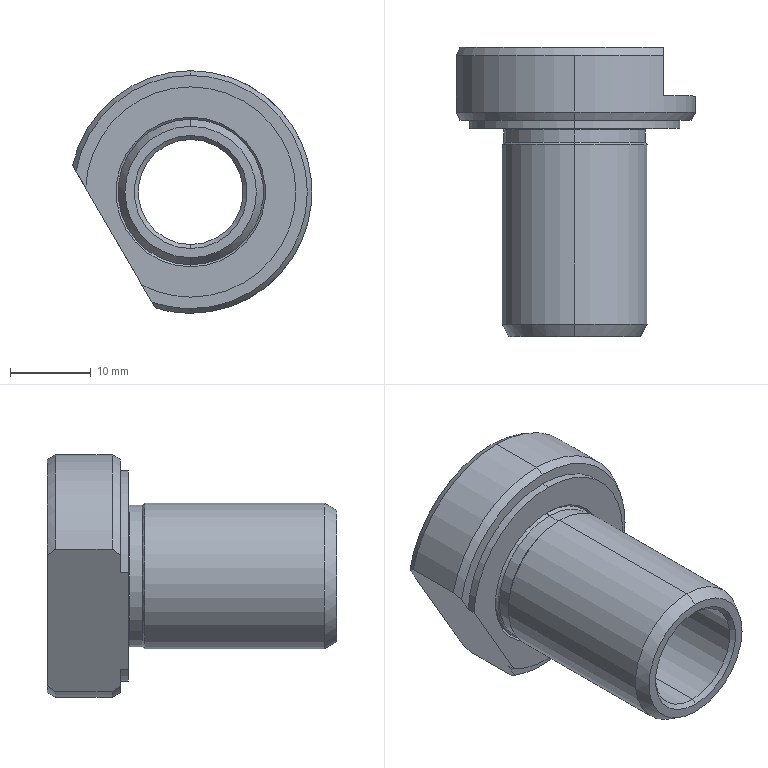Part | SolidWorks | features Chamfer 7, Cut 2, Fillet 1, Revolution 1 | 1 solid | 37 faces | box 29.63 x 35.75 x 30 mm | volume 7686 mm3 | cone 16 | cylinder 12 | plane 7 | torus 2 | commonest cylinder face diameters 26 x3 30 x3 13 x2 17.5 x2 18 x2
STEP:
#1=CARTESIAN_POINT('',(0.,-35.75,-8.134));
#2=VERTEX_POINT('',#1);
#3=CARTESIAN_POINT('',(0.,-35.75,8.134));
#4=VERTEX_POINT('',#3);
#5=CARTESIAN_POINT('',(0.,-35.75,0.));
#6=DIRECTION('',(0.,-1.,0.));
#7=DIRECTION('',(0.,0.,1.));
#8=AXIS2_PLACEMENT_3D('',#5,#6,#7);
#9=CIRCLE('',#8,8.134);
#10=EDGE_CURVE('',#2,#4,#9,.T.);
#11=ORIENTED_EDGE('',*,*,#10,.F.);
#12=CARTESIAN_POINT('',(0.,-34.25,-9.));
#13=VERTEX_POINT('',#12);
#14=CARTESIAN_POINT('',(0.,-34.25,-9.));
#15=DIRECTION('',(0.,0.866,-0.5));
#16=VECTOR('',#15,1000.);
#17=LINE('',#14,#16);
#18=EDGE_CURVE('',#2,#13,#17,.T.);
#19=ORIENTED_EDGE('',*,*,#18,.T.);
#20=CARTESIAN_POINT('',(0.,-34.25,9.));
#21=VERTEX_POINT('',#20);
#22=CARTESIAN_POINT('',(0.,-34.25,0.));
#23=DIRECTION('',(0.,1.,0.));
#24=DIRECTION('',(0.,0.,1.));
#25=AXIS2_PLACEMENT_3D('',#22,#23,#24);
#26=CIRCLE('',#25,9.);
#27=EDGE_CURVE('',#21,#13,#26,.T.);
#28=ORIENTED_EDGE('',*,*,#27,.F.);
#29=CARTESIAN_POINT('',(0.,-34.25,9.));
#30=DIRECTION('',(0.,0.866,0.5));
#31=VECTOR('',#30,1000.);
#32=LINE('',#29,#31);
#33=EDGE_CURVE('',#4,#21,#32,.T.);
#34=ORIENTED_EDGE('',*,*,#33,.F.);
#35=EDGE_LOOP('',(#11,#19,#28,#34));
#36=FACE_OUTER_BOUND('',#35,.T.);
#37=CARTESIAN_POINT('',(0.,-34.25,0.));
#38=DIRECTION('',(0.,1.,0.));
#39=DIRECTION('',(0.,0.,1.));
#40=AXIS2_PLACEMENT_3D('',#37,#38,#39);
#41=CONICAL_SURFACE('',#40,9.,0.5236);
#42=ADVANCED_FACE('',(#36),#41,.T.);
#43=CARTESIAN_POINT('',(0.,-9.75,-9.));
#44=VERTEX_POINT('',#43);
#45=CARTESIAN_POINT('',(0.,-9.75,9.));
#46=VERTEX_POINT('',#45);
#47=CARTESIAN_POINT('',(0.,-9.75,0.));
#48=DIRECTION('',(0.,1.,0.));
#49=DIRECTION('',(0.,0.,1.));
#50=AXIS2_PLACEMENT_3D('',#47,#48,#49);
#51=CIRCLE('',#50,9.);
#52=EDGE_CURVE('',#44,#46,#51,.T.);
#53=ORIENTED_EDGE('',*,*,#52,.F.);
#54=CARTESIAN_POINT('',(0.,-10.183,-8.75));
#55=VERTEX_POINT('',#54);
#56=CARTESIAN_POINT('',(0.,-10.183,-9.25));
#57=DIRECTION('',(1.,0.,0.));
#58=DIRECTION('',(0.,0.,-1.));
#59=AXIS2_PLACEMENT_3D('',#56,#57,#58);
#60=CIRCLE('',#59,0.5);
#61=EDGE_CURVE('',#44,#55,#60,.T.);
#62=ORIENTED_EDGE('',*,*,#61,.T.);
#63=CARTESIAN_POINT('',(0.,-10.183,8.75));
#64=VERTEX_POINT('',#63);
#65=CARTESIAN_POINT('',(0.,-10.183,0.));
#66=DIRECTION('',(0.,-1.,0.));
#67=DIRECTION('',(0.,0.,1.));
#68=AXIS2_PLACEMENT_3D('',#65,#66,#67);
#69=CIRCLE('',#68,8.75);
#70=EDGE_CURVE('',#64,#55,#69,.T.);
#71=ORIENTED_EDGE('',*,*,#70,.F.);
#72=CARTESIAN_POINT('',(0.,-10.183,9.25));
#73=DIRECTION('',(-1.,0.,0.));
#74=DIRECTION('',(0.,0.,1.));
#75=AXIS2_PLACEMENT_3D('',#72,#73,#74);
#76=CIRCLE('',#75,0.5);
#77=EDGE_CURVE('',#46,#64,#76,.T.);
#78=ORIENTED_EDGE('',*,*,#77,.F.);
#79=EDGE_LOOP('',(#53,#62,#71,#78));
#80=FACE_OUTER_BOUND('',#79,.T.);
#81=CARTESIAN_POINT('',(0.,-10.183,0.));
#82=DIRECTION('',(0.,1.,0.));
#83=DIRECTION('',(0.,0.,1.));
#84=AXIS2_PLACEMENT_3D('',#81,#82,#83);
#85=TOROIDAL_SURFACE('',#84,9.25,0.5);
#86=ADVANCED_FACE('',(#80),#85,.F.);
#87=ORIENTED_EDGE('',*,*,#52,.T.);
#88=CARTESIAN_POINT('',(0.,-10.,9.25));
#89=VERTEX_POINT('',#88);
#90=CARTESIAN_POINT('',(0.,-10.,9.25));
#91=DIRECTION('',(0.,-0.7071,0.7071));
#92=VECTOR('',#91,1000.);
#93=LINE('',#90,#92);
#94=EDGE_CURVE('',#46,#89,#93,.T.);
#95=ORIENTED_EDGE('',*,*,#94,.T.);
#96=CARTESIAN_POINT('',(0.,-10.,-9.25));
#97=VERTEX_POINT('',#96);
#98=CARTESIAN_POINT('',(0.,-10.,0.));
#99=DIRECTION('',(0.,1.,0.));
#100=DIRECTION('',(0.,0.,1.));
#101=AXIS2_PLACEMENT_3D('',#98,#99,#100);
#102=CIRCLE('',#101,9.25);
#103=EDGE_CURVE('',#97,#89,#102,.T.);
#104=ORIENTED_EDGE('',*,*,#103,.F.);
#105=CARTESIAN_POINT('',(0.,-10.,-9.25));
#106=DIRECTION('',(0.,-0.7071,-0.7071));
#107=VECTOR('',#106,1000.);
#108=LINE('',#105,#107);
#109=EDGE_CURVE('',#44,#97,#108,.T.);
#110=ORIENTED_EDGE('',*,*,#109,.F.);
#111=EDGE_LOOP('',(#87,#95,#104,#110));
#112=FACE_OUTER_BOUND('',#111,.T.);
#113=CARTESIAN_POINT('',(0.,-10.,0.));
#114=DIRECTION('',(0.,-1.,0.));
#115=DIRECTION('',(0.,0.,-1.));
#116=AXIS2_PLACEMENT_3D('',#113,#114,#115);
#117=CONICAL_SURFACE('',#116,9.25,0.7854);
#118=ADVANCED_FACE('',(#112),#117,.F.);
#119=CARTESIAN_POINT('',(0.,-11.75,8.75));
#120=VERTEX_POINT('',#119);
#121=CARTESIAN_POINT('',(0.,-11.75,-8.75));
#122=VERTEX_POINT('',#121);
#123=CARTESIAN_POINT('',(0.,-11.75,0.));
#124=DIRECTION('',(0.,1.,0.));
#125=DIRECTION('',(0.,0.,1.));
#126=AXIS2_PLACEMENT_3D('',#123,#124,#125);
#127=CIRCLE('',#126,8.75);
#128=EDGE_CURVE('',#120,#122,#127,.T.);
#129=ORIENTED_EDGE('',*,*,#128,.F.);
#130=CARTESIAN_POINT('',(0.,-12.,9.));
#131=VERTEX_POINT('',#130);
#132=CARTESIAN_POINT('',(0.,-11.75,8.75));
#133=DIRECTION('',(0.,-0.7071,0.7071));
#134=VECTOR('',#133,1000.);
#135=LINE('',#132,#134);
#136=EDGE_CURVE('',#120,#131,#135,.T.);
#137=ORIENTED_EDGE('',*,*,#136,.T.);
#138=CARTESIAN_POINT('',(0.,-12.,-9.));
#139=VERTEX_POINT('',#138);
#140=CARTESIAN_POINT('',(0.,-12.,0.));
#141=DIRECTION('',(0.,-1.,0.));
#142=DIRECTION('',(0.,0.,-1.));
#143=AXIS2_PLACEMENT_3D('',#140,#141,#142);
#144=CIRCLE('',#143,9.);
#145=EDGE_CURVE('',#139,#131,#144,.T.);
#146=ORIENTED_EDGE('',*,*,#145,.F.);
#147=CARTESIAN_POINT('',(0.,-11.75,-8.75));
#148=DIRECTION('',(0.,-0.7071,-0.7071));
#149=VECTOR('',#148,1000.);
#150=LINE('',#147,#149);
#151=EDGE_CURVE('',#122,#139,#150,.T.);
#152=ORIENTED_EDGE('',*,*,#151,.F.);
#153=EDGE_LOOP('',(#129,#137,#146,#152));
#154=FACE_OUTER_BOUND('',#153,.T.);
#155=CARTESIAN_POINT('',(0.,-11.75,0.));
#156=DIRECTION('',(0.,-1.,0.));
#157=DIRECTION('',(0.,0.,-1.));
#158=AXIS2_PLACEMENT_3D('',#155,#156,#157);
#159=CONICAL_SURFACE('',#158,8.75,0.7854);
#160=ADVANCED_FACE('',(#154),#159,.T.);
#161=CARTESIAN_POINT('',(0.,-35.25,6.5));
#162=VERTEX_POINT('',#161);
#163=CARTESIAN_POINT('',(0.,-35.25,-6.5));
#164=VERTEX_POINT('',#163);
#165=CARTESIAN_POINT('',(0.,-35.25,0.));
#166=DIRECTION('',(0.,-1.,0.));
#167=DIRECTION('',(0.,0.,1.));
#168=AXIS2_PLACEMENT_3D('',#165,#166,#167);
#169=CIRCLE('',#168,6.5);
#170=EDGE_CURVE('',#162,#164,#169,.T.);
#171=ORIENTED_EDGE('',*,*,#170,.F.);
#172=CARTESIAN_POINT('',(0.,-35.75,7.));
#173=VERTEX_POINT('',#172);
#174=CARTESIAN_POINT('',(0.,-35.75,7.));
#175=DIRECTION('',(0.,-0.7071,0.7071));
#176=VECTOR('',#175,1000.);
#177=LINE('',#174,#176);
#178=EDGE_CURVE('',#162,#173,#177,.T.);
#179=ORIENTED_EDGE('',*,*,#178,.T.);
#180=CARTESIAN_POINT('',(0.,-35.75,-7.));
#181=VERTEX_POINT('',#180);
#182=CARTESIAN_POINT('',(0.,-35.75,0.));
#183=DIRECTION('',(0.,1.,0.));
#184=DIRECTION('',(0.,0.,1.));
#185=AXIS2_PLACEMENT_3D('',#182,#183,#184);
#186=CIRCLE('',#185,7.);
#187=EDGE_CURVE('',#181,#173,#186,.T.);
#188=ORIENTED_EDGE('',*,*,#187,.F.);
#189=CARTESIAN_POINT('',(0.,-35.75,-7.));
#190=DIRECTION('',(0.,-0.7071,-0.7071));
#191=VECTOR('',#190,1000.);
#192=LINE('',#189,#191);
#193=EDGE_CURVE('',#164,#181,#192,.T.);
#194=ORIENTED_EDGE('',*,*,#193,.F.);
#195=EDGE_LOOP('',(#171,#179,#188,#194));
#196=FACE_OUTER_BOUND('',#195,.T.);
#197=CARTESIAN_POINT('',(0.,-35.75,0.));
#198=DIRECTION('',(0.,-1.,0.));
#199=DIRECTION('',(0.,0.,-1.));
#200=AXIS2_PLACEMENT_3D('',#197,#198,#199);
#201=CONICAL_SURFACE('',#200,7.,0.7854);
#202=ADVANCED_FACE('',(#196),#201,.F.);
#203=CARTESIAN_POINT('',(0.,-2.,-6.5));
#204=VERTEX_POINT('',#203);
#205=CARTESIAN_POINT('',(0.,-2.,6.5));
#206=VERTEX_POINT('',#205);
#207=CARTESIAN_POINT('',(0.,-2.,0.));
#208=DIRECTION('',(0.,1.,0.));
#209=DIRECTION('',(0.,0.,-1.));
#210=AXIS2_PLACEMENT_3D('',#207,#208,#209);
#211=CIRCLE('',#210,6.5);
#212=EDGE_CURVE('',#204,#206,#211,.T.);
#213=ORIENTED_EDGE('',*,*,#212,.F.);
#214=CARTESIAN_POINT('',(0.,0.,-7.655));
#215=VERTEX_POINT('',#214);
#216=CARTESIAN_POINT('',(0.,-2.,-6.5));
#217=DIRECTION('',(0.,0.866,-0.5));
#218=VECTOR('',#217,1000.);
#219=LINE('',#216,#218);
#220=EDGE_CURVE('',#204,#215,#219,.T.);
#221=ORIENTED_EDGE('',*,*,#220,.T.);
#222=CARTESIAN_POINT('',(0.,0.,7.655));
#223=VERTEX_POINT('',#222);
#224=CARTESIAN_POINT('',(0.,0.,0.));
#225=DIRECTION('',(0.,-1.,0.));
#226=DIRECTION('',(0.,0.,-1.));
#227=AXIS2_PLACEMENT_3D('',#224,#225,#226);
#228=CIRCLE('',#227,7.655);
#229=EDGE_CURVE('',#223,#215,#228,.T.);
#230=ORIENTED_EDGE('',*,*,#229,.F.);
#231=CARTESIAN_POINT('',(0.,-2.,6.5));
#232=DIRECTION('',(0.,0.866,0.5));
#233=VECTOR('',#232,1000.);
#234=LINE('',#231,#233);
#235=EDGE_CURVE('',#206,#223,#234,.T.);
#236=ORIENTED_EDGE('',*,*,#235,.F.);
#237=EDGE_LOOP('',(#213,#221,#230,#236));
#238=FACE_OUTER_BOUND('',#237,.T.);
#239=CARTESIAN_POINT('',(0.,-2.,0.));
#240=DIRECTION('',(0.,1.,0.));
#241=DIRECTION('',(0.,0.,1.));
#242=AXIS2_PLACEMENT_3D('',#239,#240,#241);
#243=CONICAL_SURFACE('',#242,6.5,0.5236);
#244=ADVANCED_FACE('',(#238),#243,.F.);
#245=ORIENTED_EDGE('',*,*,#170,.T.);
#246=CARTESIAN_POINT('',(0.,102.352,-6.5));
#247=DIRECTION('',(0.,1.,0.));
#248=VECTOR('',#247,1000.);
#249=LINE('',#246,#248);
#250=EDGE_CURVE('',#164,#204,#249,.T.);
#251=ORIENTED_EDGE('',*,*,#250,.T.);
#252=ORIENTED_EDGE('',*,*,#212,.T.);
#253=CARTESIAN_POINT('',(0.,102.352,6.5));
#254=DIRECTION('',(0.,1.,0.));
#255=VECTOR('',#254,1000.);
#256=LINE('',#253,#255);
#257=EDGE_CURVE('',#162,#206,#256,.T.);
#258=ORIENTED_EDGE('',*,*,#257,.F.);
#259=EDGE_LOOP('',(#245,#251,#252,#258));
#260=FACE_OUTER_BOUND('',#259,.T.);
#261=CARTESIAN_POINT('',(0.,102.352,0.));
#262=DIRECTION('',(0.,1.,0.));
#263=DIRECTION('',(0.,0.,1.));
#264=AXIS2_PLACEMENT_3D('',#261,#262,#263);
#265=CYLINDRICAL_SURFACE('',#264,6.5);
#266=ADVANCED_FACE('',(#260),#265,.F.);
#267=ORIENTED_EDGE('',*,*,#27,.T.);
#268=CARTESIAN_POINT('',(0.,102.352,-9.));
#269=DIRECTION('',(0.,1.,0.));
#270=VECTOR('',#269,1000.);
#271=LINE('',#268,#270);
#272=EDGE_CURVE('',#13,#139,#271,.T.);
#273=ORIENTED_EDGE('',*,*,#272,.T.);
#274=ORIENTED_EDGE('',*,*,#145,.T.);
#275=CARTESIAN_POINT('',(0.,102.352,9.));
#276=DIRECTION('',(0.,1.,0.));
#277=VECTOR('',#276,1000.);
#278=LINE('',#275,#277);
#279=EDGE_CURVE('',#21,#131,#278,.T.);
#280=ORIENTED_EDGE('',*,*,#279,.F.);
#281=EDGE_LOOP('',(#267,#273,#274,#280));
#282=FACE_OUTER_BOUND('',#281,.T.);
#283=CARTESIAN_POINT('',(0.,102.352,0.));
#284=DIRECTION('',(0.,1.,0.));
#285=DIRECTION('',(0.,0.,1.));
#286=AXIS2_PLACEMENT_3D('',#283,#284,#285);
#287=CYLINDRICAL_SURFACE('',#286,9.);
#288=ADVANCED_FACE('',(#282),#287,.T.);
#289=ORIENTED_EDGE('',*,*,#128,.T.);
#290=CARTESIAN_POINT('',(0.,102.352,-8.75));
#291=DIRECTION('',(0.,1.,0.));
#292=VECTOR('',#291,1000.);
#293=LINE('',#290,#292);
#294=EDGE_CURVE('',#122,#55,#293,.T.);
#295=ORIENTED_EDGE('',*,*,#294,.T.);
#296=CARTESIAN_POINT('',(0.,-10.183,0.));
#297=DIRECTION('',(0.,-1.,0.));
#298=DIRECTION('',(0.,0.,1.));
#299=AXIS2_PLACEMENT_3D('',#296,#297,#298);
#300=CIRCLE('',#299,8.75);
#301=EDGE_CURVE('',#55,#64,#300,.T.);
#302=ORIENTED_EDGE('',*,*,#301,.T.);
#303=CARTESIAN_POINT('',(0.,102.352,8.75));
#304=DIRECTION('',(0.,1.,0.));
#305=VECTOR('',#304,1000.);
#306=LINE('',#303,#305);
#307=EDGE_CURVE('',#120,#64,#306,.T.);
#308=ORIENTED_EDGE('',*,*,#307,.F.);
#309=EDGE_LOOP('',(#289,#295,#302,#308));
#310=FACE_OUTER_BOUND('',#309,.T.);
#311=CARTESIAN_POINT('',(0.,102.352,0.));
#312=DIRECTION('',(0.,1.,0.));
#313=DIRECTION('',(0.,0.,1.));
#314=AXIS2_PLACEMENT_3D('',#311,#312,#313);
#315=CYLINDRICAL_SURFACE('',#314,8.75);
#316=ADVANCED_FACE('',(#310),#315,.T.);
#317=CARTESIAN_POINT('',(0.,-9.,-14.423));
#318=VERTEX_POINT('',#317);
#319=CARTESIAN_POINT('',(0.,-9.,14.423));
#320=VERTEX_POINT('',#319);
#321=CARTESIAN_POINT('',(0.,-9.,0.));
#322=DIRECTION('',(0.,-1.,0.));
#323=DIRECTION('',(0.,0.,1.));
#324=AXIS2_PLACEMENT_3D('',#321,#322,#323);
#325=CIRCLE('',#324,14.423);
#326=EDGE_CURVE('',#318,#320,#325,.T.);
#327=ORIENTED_EDGE('',*,*,#326,.F.);
#328=CARTESIAN_POINT('',(0.,-8.,-15.));
#329=VERTEX_POINT('',#328);
#330=CARTESIAN_POINT('',(0.,-8.,-15.));
#331=DIRECTION('',(0.,0.866,-0.5));
#332=VECTOR('',#331,1000.);
#333=LINE('',#330,#332);
#334=EDGE_CURVE('',#318,#329,#333,.T.);
#335=ORIENTED_EDGE('',*,*,#334,.T.);
#336=CARTESIAN_POINT('',(0.,-8.,15.));
#337=VERTEX_POINT('',#336);
#338=CARTESIAN_POINT('',(0.,-8.,0.));
#339=DIRECTION('',(0.,1.,0.));
#340=DIRECTION('',(0.,0.,1.));
#341=AXIS2_PLACEMENT_3D('',#338,#339,#340);
#342=CIRCLE('',#341,15.);
#343=EDGE_CURVE('',#337,#329,#342,.T.);
#344=ORIENTED_EDGE('',*,*,#343,.F.);
#345=CARTESIAN_POINT('',(0.,-8.,15.));
#346=DIRECTION('',(0.,0.866,0.5));
#347=VECTOR('',#346,1000.);
#348=LINE('',#345,#347);
#349=EDGE_CURVE('',#320,#337,#348,.T.);
#350=ORIENTED_EDGE('',*,*,#349,.F.);
#351=EDGE_LOOP('',(#327,#335,#344,#350));
#352=FACE_OUTER_BOUND('',#351,.T.);
#353=CARTESIAN_POINT('',(0.,-8.,0.));
#354=DIRECTION('',(0.,1.,0.));
#355=DIRECTION('',(0.,0.,1.));
#356=AXIS2_PLACEMENT_3D('',#353,#354,#355);
#357=CONICAL_SURFACE('',#356,15.,0.5236);
#358=ADVANCED_FACE('',(#352),#357,.T.);
#359=CARTESIAN_POINT('',(-14.194,-9.,2.56));
#360=VERTEX_POINT('',#359);
#361=CARTESIAN_POINT('',(0.,-9.,0.));
#362=DIRECTION('',(0.,-1.,0.));
#363=DIRECTION('',(0.,0.,1.));
#364=AXIS2_PLACEMENT_3D('',#361,#362,#363);
#365=CIRCLE('',#364,14.423);
#366=EDGE_CURVE('',#320,#360,#365,.T.);
#367=ORIENTED_EDGE('',*,*,#366,.F.);
#368=ORIENTED_EDGE('',*,*,#349,.T.);
#369=CARTESIAN_POINT('',(-14.63,-8.,3.313));
#370=VERTEX_POINT('',#369);
#371=CARTESIAN_POINT('',(0.,-8.,0.));
#372=DIRECTION('',(0.,1.,0.));
#373=DIRECTION('',(0.,0.,1.));
#374=AXIS2_PLACEMENT_3D('',#371,#372,#373);
#375=CIRCLE('',#374,15.);
#376=EDGE_CURVE('',#370,#337,#375,.T.);
#377=ORIENTED_EDGE('',*,*,#376,.F.);
#378=CARTESIAN_POINT('',(-14.63,-8.,3.313));
#379=CARTESIAN_POINT('',(-14.486,-8.337,3.065));
#380=CARTESIAN_POINT('',(-14.341,-8.67,2.815));
#381=CARTESIAN_POINT('',(-14.194,-9.,2.56));
#382=B_SPLINE_CURVE_WITH_KNOTS('',3,(#378,#379,#380,#381),.UNSPECIFIED.,.F.,.F.,(4,4),(0.03086,0.03219),.UNSPECIFIED.);
#383=EDGE_CURVE('',#370,#360,#382,.T.);
#384=ORIENTED_EDGE('',*,*,#383,.T.);
#385=EDGE_LOOP('',(#367,#368,#377,#384));
#386=FACE_OUTER_BOUND('',#385,.T.);
#387=CARTESIAN_POINT('',(0.,-8.,0.));
#388=DIRECTION('',(0.,1.,0.));
#389=DIRECTION('',(0.,0.,1.));
#390=AXIS2_PLACEMENT_3D('',#387,#388,#389);
#391=CONICAL_SURFACE('',#390,15.,0.5236);
#392=ADVANCED_FACE('',(#386),#391,.T.);
#393=CARTESIAN_POINT('',(0.,-10.,13.));
#394=VERTEX_POINT('',#393);
#395=CARTESIAN_POINT('',(0.,-10.,-13.));
#396=VERTEX_POINT('',#395);
#397=CARTESIAN_POINT('',(0.,-10.,0.));
#398=DIRECTION('',(0.,1.,0.));
#399=DIRECTION('',(0.,0.,1.));
#400=AXIS2_PLACEMENT_3D('',#397,#398,#399);
#401=CIRCLE('',#400,13.);
#402=EDGE_CURVE('',#394,#396,#401,.T.);
#403=ORIENTED_EDGE('',*,*,#402,.T.);
#404=CARTESIAN_POINT('',(0.,-9.,-13.));
#405=VERTEX_POINT('',#404);
#406=CARTESIAN_POINT('',(0.,102.352,-13.));
#407=DIRECTION('',(0.,1.,0.));
#408=VECTOR('',#407,1000.);
#409=LINE('',#406,#408);
#410=EDGE_CURVE('',#396,#405,#409,.T.);
#411=ORIENTED_EDGE('',*,*,#410,.T.);
#412=CARTESIAN_POINT('',(0.,-9.,13.));
#413=VERTEX_POINT('',#412);
#414=CARTESIAN_POINT('',(0.,-9.,0.));
#415=DIRECTION('',(0.,1.,0.));
#416=DIRECTION('',(0.,0.,1.));
#417=AXIS2_PLACEMENT_3D('',#414,#415,#416);
#418=CIRCLE('',#417,13.);
#419=EDGE_CURVE('',#413,#405,#418,.T.);
#420=ORIENTED_EDGE('',*,*,#419,.F.);
#421=CARTESIAN_POINT('',(0.,102.352,13.));
#422=DIRECTION('',(0.,1.,0.));
#423=VECTOR('',#422,1000.);
#424=LINE('',#421,#423);
#425=EDGE_CURVE('',#394,#413,#424,.T.);
#426=ORIENTED_EDGE('',*,*,#425,.F.);
#427=EDGE_LOOP('',(#403,#411,#420,#426));
#428=FACE_OUTER_BOUND('',#427,.T.);
#429=CARTESIAN_POINT('',(0.,102.352,0.));
#430=DIRECTION('',(0.,1.,0.));
#431=DIRECTION('',(0.,0.,1.));
#432=AXIS2_PLACEMENT_3D('',#429,#430,#431);
#433=CYLINDRICAL_SURFACE('',#432,13.);
#434=ADVANCED_FACE('',(#428),#433,.T.);
#435=CARTESIAN_POINT('',(-12.991,-10.,0.4832));
#436=VERTEX_POINT('',#435);
#437=CARTESIAN_POINT('',(0.,-10.,0.));
#438=DIRECTION('',(0.,1.,0.));
#439=DIRECTION('',(0.,0.,1.));
#440=AXIS2_PLACEMENT_3D('',#437,#438,#439);
#441=CIRCLE('',#440,13.);
#442=EDGE_CURVE('',#436,#394,#441,.T.);
#443=ORIENTED_EDGE('',*,*,#442,.T.);
#444=ORIENTED_EDGE('',*,*,#425,.T.);
#445=CARTESIAN_POINT('',(-12.991,-9.,0.4832));
#446=VERTEX_POINT('',#445);
#447=CARTESIAN_POINT('',(0.,-9.,0.));
#448=DIRECTION('',(0.,1.,0.));
#449=DIRECTION('',(0.,0.,1.));
#450=AXIS2_PLACEMENT_3D('',#447,#448,#449);
#451=CIRCLE('',#450,13.);
#452=EDGE_CURVE('',#446,#413,#451,.T.);
#453=ORIENTED_EDGE('',*,*,#452,.F.);
#454=CARTESIAN_POINT('',(-12.991,102.352,0.4832));
#455=DIRECTION('',(0.,1.,0.));
#456=VECTOR('',#455,1000.);
#457=LINE('',#454,#456);
#458=EDGE_CURVE('',#436,#446,#457,.T.);
#459=ORIENTED_EDGE('',*,*,#458,.F.);
#460=EDGE_LOOP('',(#443,#444,#453,#459));
#461=FACE_OUTER_BOUND('',#460,.T.);
#462=CARTESIAN_POINT('',(0.,102.352,0.));
#463=DIRECTION('',(0.,1.,0.));
#464=DIRECTION('',(0.,0.,1.));
#465=AXIS2_PLACEMENT_3D('',#462,#463,#464);
#466=CYLINDRICAL_SURFACE('',#465,13.);
#467=ADVANCED_FACE('',(#461),#466,.T.);
#468=CARTESIAN_POINT('',(0.,0.,-14.423));
#469=VERTEX_POINT('',#468);
#470=CARTESIAN_POINT('',(-4.845,0.,-13.585));
#471=VERTEX_POINT('',#470);
#472=CARTESIAN_POINT('',(0.,0.,0.));
#473=DIRECTION('',(0.,1.,0.));
#474=DIRECTION('',(0.,0.,-1.));
#475=AXIS2_PLACEMENT_3D('',#472,#473,#474);
#476=CIRCLE('',#475,14.423);
#477=EDGE_CURVE('',#469,#471,#476,.T.);
#478=ORIENTED_EDGE('',*,*,#477,.F.);
#479=CARTESIAN_POINT('',(0.,-1.,-15.));
#480=VERTEX_POINT('',#479);
#481=CARTESIAN_POINT('',(0.,0.,-14.423));
#482=DIRECTION('',(0.,-0.866,-0.5));
#483=VECTOR('',#482,1000.);
#484=LINE('',#481,#483);
#485=EDGE_CURVE('',#469,#480,#484,.T.);
#486=ORIENTED_EDGE('',*,*,#485,.T.);
#487=CARTESIAN_POINT('',(-4.409,-1.,-14.337));
#488=VERTEX_POINT('',#487);
#489=CARTESIAN_POINT('',(0.,-1.,0.));
#490=DIRECTION('',(0.,-1.,0.));
#491=DIRECTION('',(0.,0.,-1.));
#492=AXIS2_PLACEMENT_3D('',#489,#490,#491);
#493=CIRCLE('',#492,15.);
#494=EDGE_CURVE('',#488,#480,#493,.T.);
#495=ORIENTED_EDGE('',*,*,#494,.F.);
#496=CARTESIAN_POINT('',(-4.409,-1.,-14.337));
#497=CARTESIAN_POINT('',(-4.552,-0.6633,-14.09));
#498=CARTESIAN_POINT('',(-4.697,-0.3298,-13.839));
#499=CARTESIAN_POINT('',(-4.845,0.,-13.585));
#500=B_SPLINE_CURVE_WITH_KNOTS('',3,(#496,#497,#498,#499),.UNSPECIFIED.,.F.,.F.,(4,4),(0.02893,0.03025),.UNSPECIFIED.);
#501=EDGE_CURVE('',#488,#471,#500,.T.);
#502=ORIENTED_EDGE('',*,*,#501,.T.);
#503=EDGE_LOOP('',(#478,#486,#495,#502));
#504=FACE_OUTER_BOUND('',#503,.T.);
#505=CARTESIAN_POINT('',(0.,0.,0.));
#506=DIRECTION('',(0.,-1.,0.));
#507=DIRECTION('',(0.,0.,-1.));
#508=AXIS2_PLACEMENT_3D('',#505,#506,#507);
#509=CONICAL_SURFACE('',#508,14.423,0.5236);
#510=ADVANCED_FACE('',(#504),#509,.T.);
#511=ORIENTED_EDGE('',*,*,#343,.T.);
#512=CARTESIAN_POINT('',(0.,102.352,-15.));
#513=DIRECTION('',(0.,1.,0.));
#514=VECTOR('',#513,1000.);
#515=LINE('',#512,#514);
#516=EDGE_CURVE('',#329,#480,#515,.T.);
#517=ORIENTED_EDGE('',*,*,#516,.T.);
#518=CARTESIAN_POINT('',(11.,-1.,-10.198));
#519=VERTEX_POINT('',#518);
#520=CARTESIAN_POINT('',(0.,-1.,0.));
#521=DIRECTION('',(0.,-1.,0.));
#522=DIRECTION('',(0.,0.,-1.));
#523=AXIS2_PLACEMENT_3D('',#520,#521,#522);
#524=CIRCLE('',#523,15.);
#525=EDGE_CURVE('',#480,#519,#524,.T.);
#526=ORIENTED_EDGE('',*,*,#525,.T.);
#527=CARTESIAN_POINT('',(11.,-6.,-10.198));
#528=VERTEX_POINT('',#527);
#529=CARTESIAN_POINT('',(11.,102.352,-10.198));
#530=DIRECTION('',(0.,1.,0.));
#531=VECTOR('',#530,1000.);
#532=LINE('',#529,#531);
#533=EDGE_CURVE('',#528,#519,#532,.T.);
#534=ORIENTED_EDGE('',*,*,#533,.F.);
#535=CARTESIAN_POINT('',(11.,-6.,10.198));
#536=VERTEX_POINT('',#535);
#537=CARTESIAN_POINT('',(0.,-6.,0.));
#538=DIRECTION('',(0.,1.,0.));
#539=DIRECTION('',(0.,0.,1.));
#540=AXIS2_PLACEMENT_3D('',#537,#538,#539);
#541=CIRCLE('',#540,15.);
#542=EDGE_CURVE('',#536,#528,#541,.T.);
#543=ORIENTED_EDGE('',*,*,#542,.F.);
#544=CARTESIAN_POINT('',(11.,-1.,10.198));
#545=VERTEX_POINT('',#544);
#546=CARTESIAN_POINT('',(11.,102.352,10.198));
#547=DIRECTION('',(0.,-1.,0.));
#548=VECTOR('',#547,1000.);
#549=LINE('',#546,#548);
#550=EDGE_CURVE('',#545,#536,#549,.T.);
#551=ORIENTED_EDGE('',*,*,#550,.F.);
#552=CARTESIAN_POINT('',(0.,-1.,15.));
#553=VERTEX_POINT('',#552);
#554=CARTESIAN_POINT('',(0.,-1.,0.));
#555=DIRECTION('',(0.,-1.,0.));
#556=DIRECTION('',(0.,0.,-1.));
#557=AXIS2_PLACEMENT_3D('',#554,#555,#556);
#558=CIRCLE('',#557,15.);
#559=EDGE_CURVE('',#545,#553,#558,.T.);
#560=ORIENTED_EDGE('',*,*,#559,.T.);
#561=CARTESIAN_POINT('',(0.,102.352,15.));
#562=DIRECTION('',(0.,1.,0.));
#563=VECTOR('',#562,1000.);
#564=LINE('',#561,#563);
#565=EDGE_CURVE('',#337,#553,#564,.T.);
#566=ORIENTED_EDGE('',*,*,#565,.F.);
#567=EDGE_LOOP('',(#511,#517,#526,#534,#543,#551,#560,#566));
#568=FACE_OUTER_BOUND('',#567,.T.);
#569=CARTESIAN_POINT('',(0.,102.352,0.));
#570=DIRECTION('',(0.,1.,0.));
#571=DIRECTION('',(0.,0.,1.));
#572=AXIS2_PLACEMENT_3D('',#569,#570,#571);
#573=CYLINDRICAL_SURFACE('',#572,15.);
#574=ADVANCED_FACE('',(#568),#573,.T.);
#575=ORIENTED_EDGE('',*,*,#376,.T.);
#576=ORIENTED_EDGE('',*,*,#565,.T.);
#577=CARTESIAN_POINT('',(-14.63,-1.,3.313));
#578=VERTEX_POINT('',#577);
#579=CARTESIAN_POINT('',(0.,-1.,0.));
#580=DIRECTION('',(0.,-1.,0.));
#581=DIRECTION('',(0.,0.,-1.));
#582=AXIS2_PLACEMENT_3D('',#579,#580,#581);
#583=CIRCLE('',#582,15.);
#584=EDGE_CURVE('',#553,#578,#583,.T.);
#585=ORIENTED_EDGE('',*,*,#584,.T.);
#586=CARTESIAN_POINT('',(-14.63,102.352,3.313));
#587=DIRECTION('',(0.,1.,0.));
#588=VECTOR('',#587,1000.);
#589=LINE('',#586,#588);
#590=EDGE_CURVE('',#370,#578,#589,.T.);
#591=ORIENTED_EDGE('',*,*,#590,.F.);
#592=EDGE_LOOP('',(#575,#576,#585,#591));
#593=FACE_OUTER_BOUND('',#592,.T.);
#594=CARTESIAN_POINT('',(0.,102.352,0.));
#595=DIRECTION('',(0.,1.,0.));
#596=DIRECTION('',(0.,0.,1.));
#597=AXIS2_PLACEMENT_3D('',#594,#595,#596);
#598=CYLINDRICAL_SURFACE('',#597,15.);
#599=ADVANCED_FACE('',(#593),#598,.T.);
#600=ORIENTED_EDGE('',*,*,#516,.F.);
#601=CARTESIAN_POINT('',(-4.409,-8.,-14.337));
#602=VERTEX_POINT('',#601);
#603=CARTESIAN_POINT('',(0.,-8.,0.));
#604=DIRECTION('',(0.,1.,0.));
#605=DIRECTION('',(0.,0.,1.));
#606=AXIS2_PLACEMENT_3D('',#603,#604,#605);
#607=CIRCLE('',#606,15.);
#608=EDGE_CURVE('',#329,#602,#607,.T.);
#609=ORIENTED_EDGE('',*,*,#608,.T.);
#610=CARTESIAN_POINT('',(-4.409,102.352,-14.337));
#611=DIRECTION('',(0.,-1.,0.));
#612=VECTOR('',#611,1000.);
#613=LINE('',#610,#612);
#614=EDGE_CURVE('',#488,#602,#613,.T.);
#615=ORIENTED_EDGE('',*,*,#614,.F.);
#616=ORIENTED_EDGE('',*,*,#494,.T.);
#617=EDGE_LOOP('',(#600,#609,#615,#616));
#618=FACE_OUTER_BOUND('',#617,.T.);
#619=CARTESIAN_POINT('',(0.,102.352,0.));
#620=DIRECTION('',(0.,1.,0.));
#621=DIRECTION('',(0.,0.,1.));
#622=AXIS2_PLACEMENT_3D('',#619,#620,#621);
#623=CYLINDRICAL_SURFACE('',#622,15.);
#624=ADVANCED_FACE('',(#618),#623,.T.);
#625=ORIENTED_EDGE('',*,*,#229,.T.);
#626=CARTESIAN_POINT('',(0.,0.,0.));
#627=DIRECTION('',(0.,-1.,0.));
#628=DIRECTION('',(0.,0.,-1.));
#629=AXIS2_PLACEMENT_3D('',#626,#627,#628);
#630=CIRCLE('',#629,7.655);
#631=EDGE_CURVE('',#215,#223,#630,.T.);
#632=ORIENTED_EDGE('',*,*,#631,.T.);
#633=EDGE_LOOP('',(#625,#632));
#634=FACE_BOUND('',#633,.T.);
#635=CARTESIAN_POINT('',(-14.194,0.,2.56));
#636=VERTEX_POINT('',#635);
#637=CARTESIAN_POINT('',(-7.887,0.,-8.331));
#638=DIRECTION('',(0.5011,0.,-0.8654));
#639=VECTOR('',#638,1000.);
#640=LINE('',#637,#639);
#641=EDGE_CURVE('',#636,#471,#640,.T.);
#642=ORIENTED_EDGE('',*,*,#641,.F.);
#643=CARTESIAN_POINT('',(11.,0.,9.328));
#644=VERTEX_POINT('',#643);
#645=CARTESIAN_POINT('',(0.,0.,0.));
#646=DIRECTION('',(0.,1.,0.));
#647=DIRECTION('',(0.,0.,-1.));
#648=AXIS2_PLACEMENT_3D('',#645,#646,#647);
#649=CIRCLE('',#648,14.423);
#650=EDGE_CURVE('',#636,#644,#649,.T.);
#651=ORIENTED_EDGE('',*,*,#650,.T.);
#652=CARTESIAN_POINT('',(11.,0.,-9.328));
#653=VERTEX_POINT('',#652);
#654=CARTESIAN_POINT('',(11.,0.,0.));
#655=DIRECTION('',(0.,0.,1.));
#656=VECTOR('',#655,1000.);
#657=LINE('',#654,#656);
#658=EDGE_CURVE('',#653,#644,#657,.T.);
#659=ORIENTED_EDGE('',*,*,#658,.F.);
#660=CARTESIAN_POINT('',(0.,0.,0.));
#661=DIRECTION('',(0.,1.,0.));
#662=DIRECTION('',(0.,0.,-1.));
#663=AXIS2_PLACEMENT_3D('',#660,#661,#662);
#664=CIRCLE('',#663,14.423);
#665=EDGE_CURVE('',#653,#469,#664,.T.);
#666=ORIENTED_EDGE('',*,*,#665,.T.);
#667=ORIENTED_EDGE('',*,*,#477,.T.);
#668=EDGE_LOOP('',(#642,#651,#659,#666,#667));
#669=FACE_OUTER_BOUND('',#668,.T.);
#670=CARTESIAN_POINT('',(6.5,0.,0.));
#671=DIRECTION('',(0.,-1.,0.));
#672=DIRECTION('',(0.,0.,-1.));
#673=AXIS2_PLACEMENT_3D('',#670,#671,#672);
#674=PLANE('',#673);
#675=ADVANCED_FACE('',(#634,#669),#674,.F.);
#676=ORIENTED_EDGE('',*,*,#485,.F.);
#677=ORIENTED_EDGE('',*,*,#665,.F.);
#678=CARTESIAN_POINT('',(11.,0.,-9.328));
#679=CARTESIAN_POINT('',(11.,-0.3297,-9.622));
#680=CARTESIAN_POINT('',(11.,-0.6633,-9.912));
#681=CARTESIAN_POINT('',(11.,-1.,-10.198));
#682=B_SPLINE_CURVE_WITH_KNOTS('',3,(#678,#679,#680,#681),.UNSPECIFIED.,.F.,.F.,(4,4),(0.04608,0.04741),.UNSPECIFIED.);
#683=EDGE_CURVE('',#653,#519,#682,.T.);
#684=ORIENTED_EDGE('',*,*,#683,.T.);
#685=ORIENTED_EDGE('',*,*,#525,.F.);
#686=EDGE_LOOP('',(#676,#677,#684,#685));
#687=FACE_OUTER_BOUND('',#686,.T.);
#688=CARTESIAN_POINT('',(0.,0.,0.));
#689=DIRECTION('',(0.,-1.,0.));
#690=DIRECTION('',(0.,0.,-1.));
#691=AXIS2_PLACEMENT_3D('',#688,#689,#690);
#692=CONICAL_SURFACE('',#691,14.423,0.5236);
#693=ADVANCED_FACE('',(#687),#692,.T.);
#694=ORIENTED_EDGE('',*,*,#650,.F.);
#695=CARTESIAN_POINT('',(-14.194,0.,2.56));
#696=CARTESIAN_POINT('',(-14.341,-0.3296,2.815));
#697=CARTESIAN_POINT('',(-14.486,-0.6632,3.065));
#698=CARTESIAN_POINT('',(-14.63,-1.,3.313));
#699=B_SPLINE_CURVE_WITH_KNOTS('',3,(#695,#696,#697,#698),.UNSPECIFIED.,.F.,.F.,(4,4),(0.053,0.05435),.UNSPECIFIED.);
#700=EDGE_CURVE('',#636,#578,#699,.T.);
#701=ORIENTED_EDGE('',*,*,#700,.T.);
#702=ORIENTED_EDGE('',*,*,#584,.F.);
#703=ORIENTED_EDGE('',*,*,#559,.F.);
#704=CARTESIAN_POINT('',(11.,-1.,10.198));
#705=CARTESIAN_POINT('',(11.,-0.6634,9.912));
#706=CARTESIAN_POINT('',(11.,-0.3299,9.623));
#707=CARTESIAN_POINT('',(11.,0.,9.328));
#708=B_SPLINE_CURVE_WITH_KNOTS('',3,(#704,#705,#706,#707),.UNSPECIFIED.,.F.,.F.,(4,4),(0.02205,0.02338),.UNSPECIFIED.);
#709=EDGE_CURVE('',#545,#644,#708,.T.);
#710=ORIENTED_EDGE('',*,*,#709,.T.);
#711=EDGE_LOOP('',(#694,#701,#702,#703,#710));
#712=FACE_OUTER_BOUND('',#711,.T.);
#713=CARTESIAN_POINT('',(0.,0.,0.));
#714=DIRECTION('',(0.,-1.,0.));
#715=DIRECTION('',(0.,0.,-1.));
#716=AXIS2_PLACEMENT_3D('',#713,#714,#715);
#717=CONICAL_SURFACE('',#716,14.423,0.5236);
#718=ADVANCED_FACE('',(#712),#717,.T.);
#719=CARTESIAN_POINT('',(-4.845,-9.,-13.585));
#720=VERTEX_POINT('',#719);
#721=CARTESIAN_POINT('',(-6.047,-9.,-11.508));
#722=VERTEX_POINT('',#721);
#723=CARTESIAN_POINT('',(-5.752,-9.,-12.017));
#724=DIRECTION('',(-0.5011,0.,0.8654));
#725=VECTOR('',#724,1000.);
#726=LINE('',#723,#725);
#727=EDGE_CURVE('',#720,#722,#726,.T.);
#728=ORIENTED_EDGE('',*,*,#727,.F.);
#729=CARTESIAN_POINT('',(0.,-9.,0.));
#730=DIRECTION('',(0.,-1.,0.));
#731=DIRECTION('',(0.,0.,1.));
#732=AXIS2_PLACEMENT_3D('',#729,#730,#731);
#733=CIRCLE('',#732,14.423);
#734=EDGE_CURVE('',#720,#318,#733,.T.);
#735=ORIENTED_EDGE('',*,*,#734,.T.);
#736=ORIENTED_EDGE('',*,*,#326,.T.);
#737=ORIENTED_EDGE('',*,*,#366,.T.);
#738=CARTESIAN_POINT('',(-5.752,-9.,-12.017));
#739=DIRECTION('',(-0.5011,0.,0.8654));
#740=VECTOR('',#739,1000.);
#741=LINE('',#738,#740);
#742=EDGE_CURVE('',#446,#360,#741,.T.);
#743=ORIENTED_EDGE('',*,*,#742,.F.);
#744=ORIENTED_EDGE('',*,*,#452,.T.);
#745=ORIENTED_EDGE('',*,*,#419,.T.);
#746=CARTESIAN_POINT('',(0.,-9.,0.));
#747=DIRECTION('',(0.,1.,0.));
#748=DIRECTION('',(0.,0.,1.));
#749=AXIS2_PLACEMENT_3D('',#746,#747,#748);
#750=CIRCLE('',#749,13.);
#751=EDGE_CURVE('',#405,#722,#750,.T.);
#752=ORIENTED_EDGE('',*,*,#751,.T.);
#753=EDGE_LOOP('',(#728,#735,#736,#737,#743,#744,#745,#752));
#754=FACE_OUTER_BOUND('',#753,.T.);
#755=CARTESIAN_POINT('',(15.,-9.,0.));
#756=DIRECTION('',(0.,1.,0.));
#757=DIRECTION('',(0.,0.,1.));
#758=AXIS2_PLACEMENT_3D('',#755,#756,#757);
#759=PLANE('',#758);
#760=ADVANCED_FACE('',(#754),#759,.F.);
#761=ORIENTED_EDGE('',*,*,#410,.F.);
#762=CARTESIAN_POINT('',(-6.047,-10.,-11.508));
#763=VERTEX_POINT('',#762);
#764=CARTESIAN_POINT('',(0.,-10.,0.));
#765=DIRECTION('',(0.,1.,0.));
#766=DIRECTION('',(0.,0.,1.));
#767=AXIS2_PLACEMENT_3D('',#764,#765,#766);
#768=CIRCLE('',#767,13.);
#769=EDGE_CURVE('',#396,#763,#768,.T.);
#770=ORIENTED_EDGE('',*,*,#769,.T.);
#771=CARTESIAN_POINT('',(-6.047,102.352,-11.508));
#772=DIRECTION('',(0.,-1.,0.));
#773=VECTOR('',#772,1000.);
#774=LINE('',#771,#773);
#775=EDGE_CURVE('',#722,#763,#774,.T.);
#776=ORIENTED_EDGE('',*,*,#775,.F.);
#777=ORIENTED_EDGE('',*,*,#751,.F.);
#778=EDGE_LOOP('',(#761,#770,#776,#777));
#779=FACE_OUTER_BOUND('',#778,.T.);
#780=CARTESIAN_POINT('',(0.,102.352,0.));
#781=DIRECTION('',(0.,1.,0.));
#782=DIRECTION('',(0.,0.,1.));
#783=AXIS2_PLACEMENT_3D('',#780,#781,#782);
#784=CYLINDRICAL_SURFACE('',#783,13.);
#785=ADVANCED_FACE('',(#779),#784,.T.);
#786=ORIENTED_EDGE('',*,*,#103,.T.);
#787=CARTESIAN_POINT('',(0.,-10.,0.));
#788=DIRECTION('',(0.,1.,0.));
#789=DIRECTION('',(0.,0.,1.));
#790=AXIS2_PLACEMENT_3D('',#787,#788,#789);
#791=CIRCLE('',#790,9.25);
#792=EDGE_CURVE('',#89,#97,#791,.T.);
#793=ORIENTED_EDGE('',*,*,#792,.T.);
#794=EDGE_LOOP('',(#786,#793));
#795=FACE_BOUND('',#794,.T.);
#796=CARTESIAN_POINT('',(-6.255,-10.,-11.15));
#797=DIRECTION('',(-0.5011,0.,0.8654));
#798=VECTOR('',#797,1000.);
#799=LINE('',#796,#798);
#800=EDGE_CURVE('',#763,#436,#799,.T.);
#801=ORIENTED_EDGE('',*,*,#800,.F.);
#802=ORIENTED_EDGE('',*,*,#769,.F.);
#803=ORIENTED_EDGE('',*,*,#402,.F.);
#804=ORIENTED_EDGE('',*,*,#442,.F.);
#805=EDGE_LOOP('',(#801,#802,#803,#804));
#806=FACE_OUTER_BOUND('',#805,.T.);
#807=CARTESIAN_POINT('',(13.,-10.,0.));
#808=DIRECTION('',(0.,1.,0.));
#809=DIRECTION('',(0.,0.,1.));
#810=AXIS2_PLACEMENT_3D('',#807,#808,#809);
#811=PLANE('',#810);
#812=ADVANCED_FACE('',(#795,#806),#811,.F.);
#813=ORIENTED_EDGE('',*,*,#334,.F.);
#814=ORIENTED_EDGE('',*,*,#734,.F.);
#815=CARTESIAN_POINT('',(-4.845,-9.,-13.585));
#816=CARTESIAN_POINT('',(-4.697,-8.671,-13.839));
#817=CARTESIAN_POINT('',(-4.552,-8.337,-14.09));
#818=CARTESIAN_POINT('',(-4.409,-8.,-14.337));
#819=B_SPLINE_CURVE_WITH_KNOTS('',3,(#815,#816,#817,#818),.UNSPECIFIED.,.F.,.F.,(4,4),(0.05482,0.05614),.UNSPECIFIED.);
#820=EDGE_CURVE('',#720,#602,#819,.T.);
#821=ORIENTED_EDGE('',*,*,#820,.T.);
#822=ORIENTED_EDGE('',*,*,#608,.F.);
#823=EDGE_LOOP('',(#813,#814,#821,#822));
#824=FACE_OUTER_BOUND('',#823,.T.);
#825=CARTESIAN_POINT('',(0.,-8.,0.));
#826=DIRECTION('',(0.,1.,0.));
#827=DIRECTION('',(0.,0.,1.));
#828=AXIS2_PLACEMENT_3D('',#825,#826,#827);
#829=CONICAL_SURFACE('',#828,15.,0.5236);
#830=ADVANCED_FACE('',(#824),#829,.T.);
#831=ORIENTED_EDGE('',*,*,#294,.F.);
#832=CARTESIAN_POINT('',(0.,-11.75,0.));
#833=DIRECTION('',(0.,1.,0.));
#834=DIRECTION('',(0.,0.,1.));
#835=AXIS2_PLACEMENT_3D('',#832,#833,#834);
#836=CIRCLE('',#835,8.75);
#837=EDGE_CURVE('',#122,#120,#836,.T.);
#838=ORIENTED_EDGE('',*,*,#837,.T.);
#839=ORIENTED_EDGE('',*,*,#307,.T.);
#840=ORIENTED_EDGE('',*,*,#70,.T.);
#841=EDGE_LOOP('',(#831,#838,#839,#840));
#842=FACE_OUTER_BOUND('',#841,.T.);
#843=CARTESIAN_POINT('',(0.,102.352,0.));
#844=DIRECTION('',(0.,1.,0.));
#845=DIRECTION('',(0.,0.,1.));
#846=AXIS2_PLACEMENT_3D('',#843,#844,#845);
#847=CYLINDRICAL_SURFACE('',#846,8.75);
#848=ADVANCED_FACE('',(#842),#847,.T.);
#849=ORIENTED_EDGE('',*,*,#272,.F.);
#850=CARTESIAN_POINT('',(0.,-34.25,0.));
#851=DIRECTION('',(0.,1.,0.));
#852=DIRECTION('',(0.,0.,1.));
#853=AXIS2_PLACEMENT_3D('',#850,#851,#852);
#854=CIRCLE('',#853,9.);
#855=EDGE_CURVE('',#13,#21,#854,.T.);
#856=ORIENTED_EDGE('',*,*,#855,.T.);
#857=ORIENTED_EDGE('',*,*,#279,.T.);
#858=CARTESIAN_POINT('',(0.,-12.,0.));
#859=DIRECTION('',(0.,-1.,0.));
#860=DIRECTION('',(0.,0.,-1.));
#861=AXIS2_PLACEMENT_3D('',#858,#859,#860);
#862=CIRCLE('',#861,9.);
#863=EDGE_CURVE('',#131,#139,#862,.T.);
#864=ORIENTED_EDGE('',*,*,#863,.T.);
#865=EDGE_LOOP('',(#849,#856,#857,#864));
#866=FACE_OUTER_BOUND('',#865,.T.);
#867=CARTESIAN_POINT('',(0.,102.352,0.));
#868=DIRECTION('',(0.,1.,0.));
#869=DIRECTION('',(0.,0.,1.));
#870=AXIS2_PLACEMENT_3D('',#867,#868,#869);
#871=CYLINDRICAL_SURFACE('',#870,9.);
#872=ADVANCED_FACE('',(#866),#871,.T.);
#873=CARTESIAN_POINT('',(0.,-35.75,0.));
#874=DIRECTION('',(0.,-1.,0.));
#875=DIRECTION('',(0.,0.,1.));
#876=AXIS2_PLACEMENT_3D('',#873,#874,#875);
#877=CIRCLE('',#876,8.134);
#878=EDGE_CURVE('',#4,#2,#877,.T.);
#879=ORIENTED_EDGE('',*,*,#878,.T.);
#880=ORIENTED_EDGE('',*,*,#10,.T.);
#881=EDGE_LOOP('',(#879,#880));
#882=FACE_OUTER_BOUND('',#881,.T.);
#883=ORIENTED_EDGE('',*,*,#187,.T.);
#884=CARTESIAN_POINT('',(0.,-35.75,0.));
#885=DIRECTION('',(0.,1.,0.));
#886=DIRECTION('',(0.,0.,1.));
#887=AXIS2_PLACEMENT_3D('',#884,#885,#886);
#888=CIRCLE('',#887,7.);
#889=EDGE_CURVE('',#173,#181,#888,.T.);
#890=ORIENTED_EDGE('',*,*,#889,.T.);
#891=EDGE_LOOP('',(#883,#890));
#892=FACE_BOUND('',#891,.T.);
#893=CARTESIAN_POINT('',(9.,-35.75,0.));
#894=DIRECTION('',(0.,1.,0.));
#895=DIRECTION('',(0.,0.,1.));
#896=AXIS2_PLACEMENT_3D('',#893,#894,#895);
#897=PLANE('',#896);
#898=ADVANCED_FACE('',(#882,#892),#897,.F.);
#899=ORIENTED_EDGE('',*,*,#250,.F.);
#900=CARTESIAN_POINT('',(0.,-35.25,0.));
#901=DIRECTION('',(0.,-1.,0.));
#902=DIRECTION('',(0.,0.,1.));
#903=AXIS2_PLACEMENT_3D('',#900,#901,#902);
#904=CIRCLE('',#903,6.5);
#905=EDGE_CURVE('',#164,#162,#904,.T.);
#906=ORIENTED_EDGE('',*,*,#905,.T.);
#907=ORIENTED_EDGE('',*,*,#257,.T.);
#908=CARTESIAN_POINT('',(0.,-2.,0.));
#909=DIRECTION('',(0.,1.,0.));
#910=DIRECTION('',(0.,0.,-1.));
#911=AXIS2_PLACEMENT_3D('',#908,#909,#910);
#912=CIRCLE('',#911,6.5);
#913=EDGE_CURVE('',#206,#204,#912,.T.);
#914=ORIENTED_EDGE('',*,*,#913,.T.);
#915=EDGE_LOOP('',(#899,#906,#907,#914));
#916=FACE_OUTER_BOUND('',#915,.T.);
#917=CARTESIAN_POINT('',(0.,102.352,0.));
#918=DIRECTION('',(0.,1.,0.));
#919=DIRECTION('',(0.,0.,1.));
#920=AXIS2_PLACEMENT_3D('',#917,#918,#919);
#921=CYLINDRICAL_SURFACE('',#920,6.5);
#922=ADVANCED_FACE('',(#916),#921,.F.);
#923=ORIENTED_EDGE('',*,*,#220,.F.);
#924=ORIENTED_EDGE('',*,*,#913,.F.);
#925=ORIENTED_EDGE('',*,*,#235,.T.);
#926=ORIENTED_EDGE('',*,*,#631,.F.);
#927=EDGE_LOOP('',(#923,#924,#925,#926));
#928=FACE_OUTER_BOUND('',#927,.T.);
#929=CARTESIAN_POINT('',(0.,-2.,0.));
#930=DIRECTION('',(0.,1.,0.));
#931=DIRECTION('',(0.,0.,1.));
#932=AXIS2_PLACEMENT_3D('',#929,#930,#931);
#933=CONICAL_SURFACE('',#932,6.5,0.5236);
#934=ADVANCED_FACE('',(#928),#933,.F.);
#935=ORIENTED_EDGE('',*,*,#178,.F.);
#936=ORIENTED_EDGE('',*,*,#905,.F.);
#937=ORIENTED_EDGE('',*,*,#193,.T.);
#938=ORIENTED_EDGE('',*,*,#889,.F.);
#939=EDGE_LOOP('',(#935,#936,#937,#938));
#940=FACE_OUTER_BOUND('',#939,.T.);
#941=CARTESIAN_POINT('',(0.,-35.75,0.));
#942=DIRECTION('',(0.,-1.,0.));
#943=DIRECTION('',(0.,0.,-1.));
#944=AXIS2_PLACEMENT_3D('',#941,#942,#943);
#945=CONICAL_SURFACE('',#944,7.,0.7854);
#946=ADVANCED_FACE('',(#940),#945,.F.);
#947=ORIENTED_EDGE('',*,*,#136,.F.);
#948=ORIENTED_EDGE('',*,*,#837,.F.);
#949=ORIENTED_EDGE('',*,*,#151,.T.);
#950=ORIENTED_EDGE('',*,*,#863,.F.);
#951=EDGE_LOOP('',(#947,#948,#949,#950));
#952=FACE_OUTER_BOUND('',#951,.T.);
#953=CARTESIAN_POINT('',(0.,-11.75,0.));
#954=DIRECTION('',(0.,-1.,0.));
#955=DIRECTION('',(0.,0.,-1.));
#956=AXIS2_PLACEMENT_3D('',#953,#954,#955);
#957=CONICAL_SURFACE('',#956,8.75,0.7854);
#958=ADVANCED_FACE('',(#952),#957,.T.);
#959=ORIENTED_EDGE('',*,*,#94,.F.);
#960=CARTESIAN_POINT('',(0.,-9.75,0.));
#961=DIRECTION('',(0.,1.,0.));
#962=DIRECTION('',(0.,0.,1.));
#963=AXIS2_PLACEMENT_3D('',#960,#961,#962);
#964=CIRCLE('',#963,9.);
#965=EDGE_CURVE('',#46,#44,#964,.T.);
#966=ORIENTED_EDGE('',*,*,#965,.T.);
#967=ORIENTED_EDGE('',*,*,#109,.T.);
#968=ORIENTED_EDGE('',*,*,#792,.F.);
#969=EDGE_LOOP('',(#959,#966,#967,#968));
#970=FACE_OUTER_BOUND('',#969,.T.);
#971=CARTESIAN_POINT('',(0.,-10.,0.));
#972=DIRECTION('',(0.,-1.,0.));
#973=DIRECTION('',(0.,0.,-1.));
#974=AXIS2_PLACEMENT_3D('',#971,#972,#973);
#975=CONICAL_SURFACE('',#974,9.25,0.7854);
#976=ADVANCED_FACE('',(#970),#975,.F.);
#977=ORIENTED_EDGE('',*,*,#61,.F.);
#978=ORIENTED_EDGE('',*,*,#965,.F.);
#979=ORIENTED_EDGE('',*,*,#77,.T.);
#980=ORIENTED_EDGE('',*,*,#301,.F.);
#981=EDGE_LOOP('',(#977,#978,#979,#980));
#982=FACE_OUTER_BOUND('',#981,.T.);
#983=CARTESIAN_POINT('',(0.,-10.183,0.));
#984=DIRECTION('',(0.,1.,0.));
#985=DIRECTION('',(0.,0.,1.));
#986=AXIS2_PLACEMENT_3D('',#983,#984,#985);
#987=TOROIDAL_SURFACE('',#986,9.25,0.5);
#988=ADVANCED_FACE('',(#982),#987,.F.);
#989=ORIENTED_EDGE('',*,*,#18,.F.);
#990=ORIENTED_EDGE('',*,*,#878,.F.);
#991=ORIENTED_EDGE('',*,*,#33,.T.);
#992=ORIENTED_EDGE('',*,*,#855,.F.);
#993=EDGE_LOOP('',(#989,#990,#991,#992));
#994=FACE_OUTER_BOUND('',#993,.T.);
#995=CARTESIAN_POINT('',(0.,-34.25,0.));
#996=DIRECTION('',(0.,1.,0.));
#997=DIRECTION('',(0.,0.,1.));
#998=AXIS2_PLACEMENT_3D('',#995,#996,#997);
#999=CONICAL_SURFACE('',#998,9.,0.5236);
#1000=ADVANCED_FACE('',(#994),#999,.T.);
#1001=CARTESIAN_POINT('',(11.,-6.,88.1));
#1002=DIRECTION('',(0.,0.,-1.));
#1003=VECTOR('',#1002,1000.);
#1004=LINE('',#1001,#1003);
#1005=EDGE_CURVE('',#536,#528,#1004,.T.);
#1006=ORIENTED_EDGE('',*,*,#1005,.F.);
#1007=ORIENTED_EDGE('',*,*,#542,.T.);
#1008=EDGE_LOOP('',(#1006,#1007));
#1009=FACE_OUTER_BOUND('',#1008,.T.);
#1010=CARTESIAN_POINT('',(11.,-6.,88.1));
#1011=DIRECTION('',(0.,1.,0.));
#1012=DIRECTION('',(0.,0.,1.));
#1013=AXIS2_PLACEMENT_3D('',#1010,#1011,#1012);
#1014=PLANE('',#1013);
#1015=ADVANCED_FACE('',(#1009),#1014,.T.);
#1016=ORIENTED_EDGE('',*,*,#709,.F.);
#1017=ORIENTED_EDGE('',*,*,#550,.T.);
#1018=ORIENTED_EDGE('',*,*,#1005,.T.);
#1019=ORIENTED_EDGE('',*,*,#533,.T.);
#1020=ORIENTED_EDGE('',*,*,#683,.F.);
#1021=ORIENTED_EDGE('',*,*,#658,.T.);
#1022=EDGE_LOOP('',(#1016,#1017,#1018,#1019,#1020,#1021));
#1023=FACE_OUTER_BOUND('',#1022,.T.);
#1024=CARTESIAN_POINT('',(11.,95.,88.1));
#1025=DIRECTION('',(1.,0.,0.));
#1026=DIRECTION('',(0.,1.,0.));
#1027=AXIS2_PLACEMENT_3D('',#1024,#1025,#1026);
#1028=PLANE('',#1027);
#1029=ADVANCED_FACE('',(#1023),#1028,.T.);
#1030=ORIENTED_EDGE('',*,*,#383,.F.);
#1031=ORIENTED_EDGE('',*,*,#590,.T.);
#1032=ORIENTED_EDGE('',*,*,#700,.F.);
#1033=ORIENTED_EDGE('',*,*,#641,.T.);
#1034=ORIENTED_EDGE('',*,*,#501,.F.);
#1035=ORIENTED_EDGE('',*,*,#614,.T.);
#1036=ORIENTED_EDGE('',*,*,#820,.F.);
#1037=ORIENTED_EDGE('',*,*,#727,.T.);
#1038=ORIENTED_EDGE('',*,*,#775,.T.);
#1039=ORIENTED_EDGE('',*,*,#800,.T.);
#1040=ORIENTED_EDGE('',*,*,#458,.T.);
#1041=ORIENTED_EDGE('',*,*,#742,.T.);
#1042=EDGE_LOOP('',(#1030,#1031,#1032,#1033,#1034,#1035,#1036,#1037,#1038,#1039,#1040,#1041));
#1043=FACE_OUTER_BOUND('',#1042,.T.);
#1044=CARTESIAN_POINT('',(-50.825,79.35,65.818));
#1045=DIRECTION('',(-0.8654,0.,-0.5011));
#1046=DIRECTION('',(-0.5011,0.,0.8654));
#1047=AXIS2_PLACEMENT_3D('',#1044,#1045,#1046);
#1048=PLANE('',#1047);
#1049=ADVANCED_FACE('',(#1043),#1048,.T.);
#1050=CLOSED_SHELL('',(#42,#86,#118,#160,#202,#244,#266,#288,#316,#358,#392,#434,#467,#510,#574,#599,#624,#675,#693,#718,#760,#785,#812,#830,#848,#872,#898,#922,#934,#946,#958,#976,#988,#1000,#1015,#1029,#1049));
#1051=MANIFOLD_SOLID_BREP('',#1050);
#1052=CARTESIAN_POINT('',(0.,0.,0.));
#1053=DIRECTION('',(0.,0.,1.));
#1054=DIRECTION('',(1.,0.,0.));
#1055=AXIS2_PLACEMENT_3D('',#1052,#1053,#1054);
#1056=(LENGTH_UNIT()NAMED_UNIT(*)SI_UNIT(.MILLI.,.METRE.));
#1057=UNCERTAINTY_MEASURE_WITH_UNIT(LENGTH_MEASURE(0.00001),#1056,'','');
#1058=(NAMED_UNIT(*)PLANE_ANGLE_UNIT()SI_UNIT($,.RADIAN.));
#1059=(NAMED_UNIT(*)SI_UNIT($,.STERADIAN.)SOLID_ANGLE_UNIT());
#1060=(GEOMETRIC_REPRESENTATION_CONTEXT(3)GLOBAL_UNCERTAINTY_ASSIGNED_CONTEXT((#1057))GLOBAL_UNIT_ASSIGNED_CONTEXT((#1056,#1058,#1059))REPRESENTATION_CONTEXT('',''));
#1061=ADVANCED_BREP_SHAPE_REPRESENTATION('',(#1051,#1055),#1060);